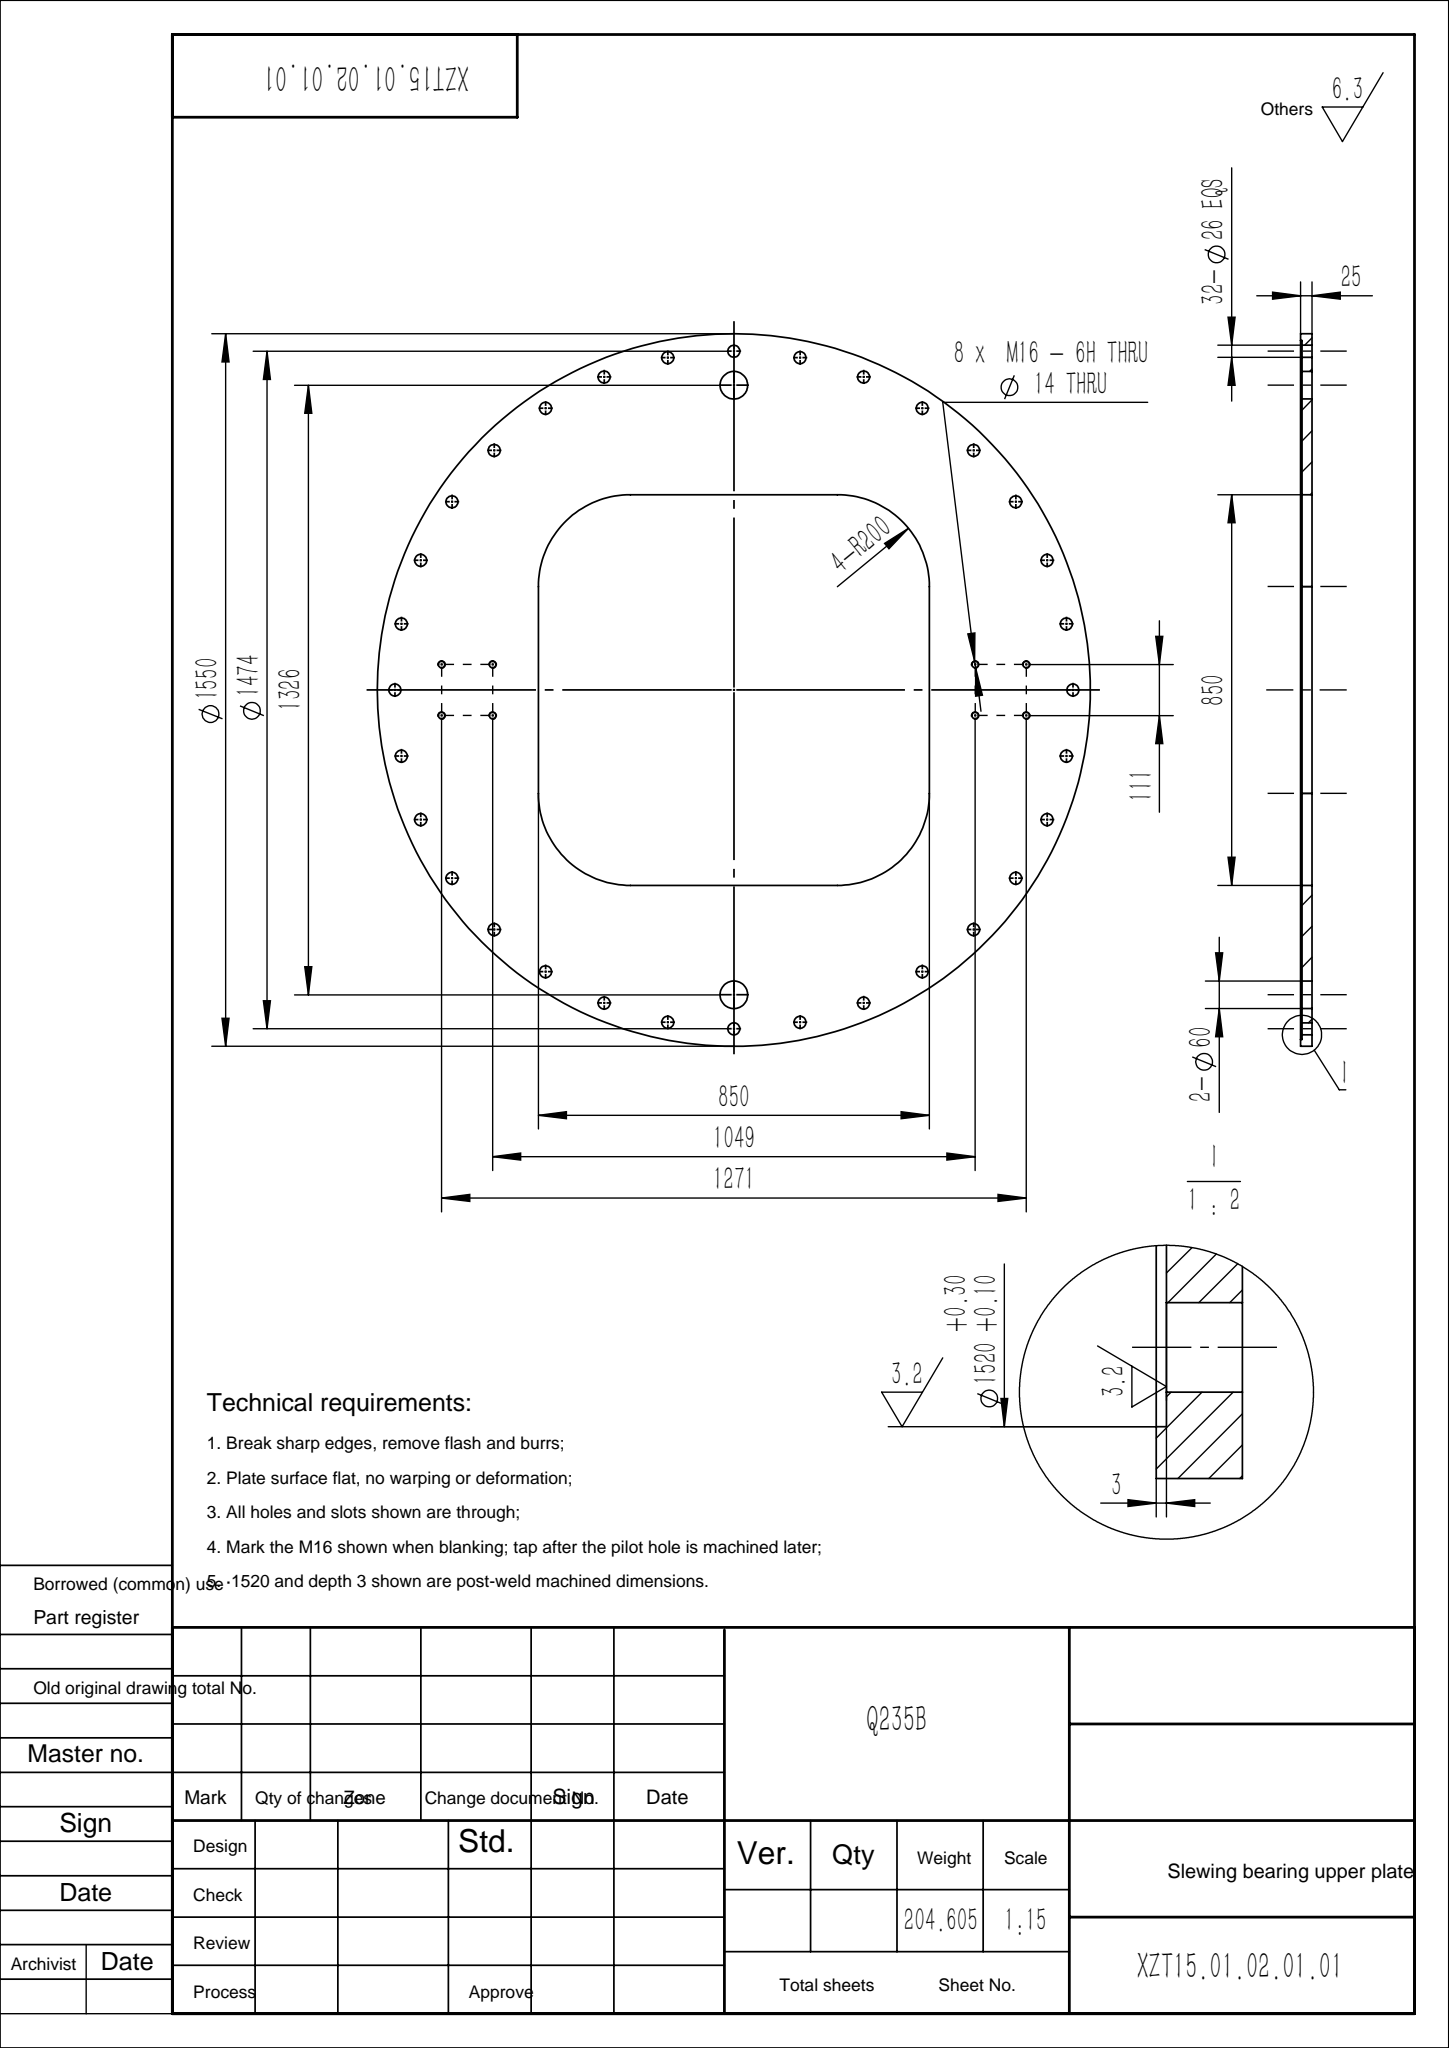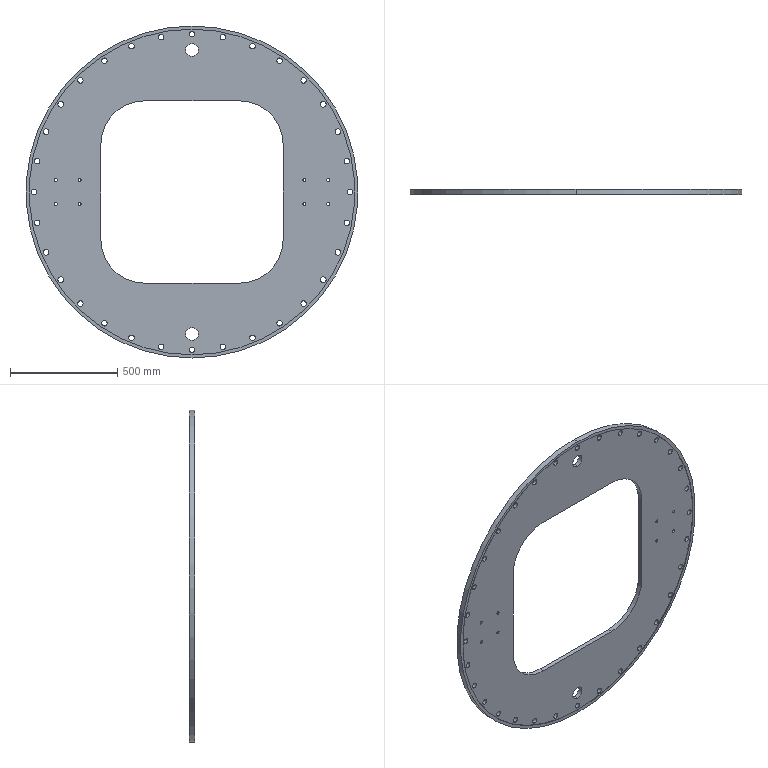Part | SolidWorks | features Extrusion 1, HoleWzd 1, ICE 1 | 1 solid | 99 faces | box 1550 x 25 x 1550 mm | volume 26064350 mm3 | cylinder 92 | plane 7 | commonest cylinder face diameters 26 x64 14 x16 60 x4 400 x4 1520 x2 1550 x2